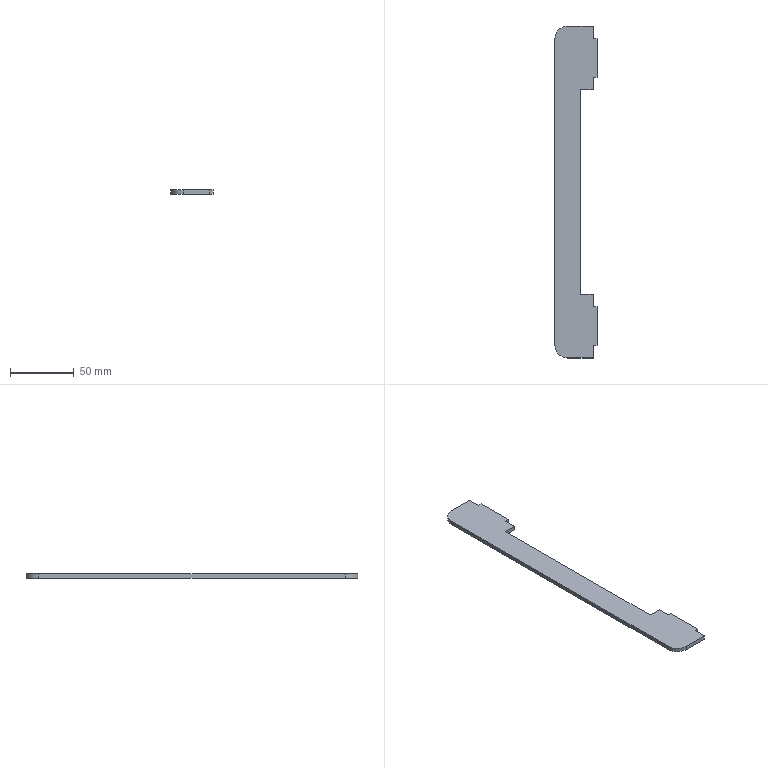Part | SolidWorks | features FlatPattern 1, SMBaseFlange 1, SheetMetal 1 | 1 solid | 20 faces | box 33 x 260 x 3.2 mm | volume 20279 mm3 | plane 18 | cylinder 2 | commonest cylinder face diameters 20 x2
STEP:
#1=CARTESIAN_POINT('',(-95.497,69.865,0.));
#2=VERTEX_POINT('',#1);
#3=CARTESIAN_POINT('',(-95.497,79.865,0.));
#4=VERTEX_POINT('',#3);
#5=CARTESIAN_POINT('',(-95.497,79.865,0.));
#6=DIRECTION('',(0.,1.,0.));
#7=VECTOR('',#6,1000.);
#8=LINE('',#5,#7);
#9=EDGE_CURVE('',#2,#4,#8,.T.);
#10=ORIENTED_EDGE('',*,*,#9,.F.);
#11=CARTESIAN_POINT('',(-95.497,69.865,-3.2));
#12=VERTEX_POINT('',#11);
#13=CARTESIAN_POINT('',(-95.497,69.865,-3.2));
#14=DIRECTION('',(0.,0.,1.));
#15=VECTOR('',#14,1000.);
#16=LINE('',#13,#15);
#17=EDGE_CURVE('',#12,#2,#16,.T.);
#18=ORIENTED_EDGE('',*,*,#17,.F.);
#19=CARTESIAN_POINT('',(-95.497,79.865,-3.2));
#20=VERTEX_POINT('',#19);
#21=CARTESIAN_POINT('',(-95.497,79.865,-3.2));
#22=DIRECTION('',(0.,1.,0.));
#23=VECTOR('',#22,1000.);
#24=LINE('',#21,#23);
#25=EDGE_CURVE('',#12,#20,#24,.T.);
#26=ORIENTED_EDGE('',*,*,#25,.T.);
#27=CARTESIAN_POINT('',(-95.497,79.865,-3.2));
#28=DIRECTION('',(0.,0.,1.));
#29=VECTOR('',#28,1000.);
#30=LINE('',#27,#29);
#31=EDGE_CURVE('',#20,#4,#30,.T.);
#32=ORIENTED_EDGE('',*,*,#31,.T.);
#33=EDGE_LOOP('',(#10,#18,#26,#32));
#34=FACE_OUTER_BOUND('',#33,.T.);
#35=CARTESIAN_POINT('',(-95.497,79.865,-3.2));
#36=DIRECTION('',(1.,0.,0.));
#37=DIRECTION('',(0.,0.,-1.));
#38=AXIS2_PLACEMENT_3D('',#35,#36,#37);
#39=PLANE('',#38);
#40=ADVANCED_FACE('',(#34),#39,.T.);
#41=CARTESIAN_POINT('',(-105.497,69.865,0.));
#42=VERTEX_POINT('',#41);
#43=CARTESIAN_POINT('',(-95.497,69.865,0.));
#44=DIRECTION('',(1.,0.,0.));
#45=VECTOR('',#44,1000.);
#46=LINE('',#43,#45);
#47=EDGE_CURVE('',#42,#2,#46,.T.);
#48=ORIENTED_EDGE('',*,*,#47,.F.);
#49=CARTESIAN_POINT('',(-105.497,69.865,-3.2));
#50=VERTEX_POINT('',#49);
#51=CARTESIAN_POINT('',(-105.497,69.865,-3.2));
#52=DIRECTION('',(0.,0.,1.));
#53=VECTOR('',#52,1000.);
#54=LINE('',#51,#53);
#55=EDGE_CURVE('',#50,#42,#54,.T.);
#56=ORIENTED_EDGE('',*,*,#55,.F.);
#57=CARTESIAN_POINT('',(-95.497,69.865,-3.2));
#58=DIRECTION('',(1.,0.,0.));
#59=VECTOR('',#58,1000.);
#60=LINE('',#57,#59);
#61=EDGE_CURVE('',#50,#12,#60,.T.);
#62=ORIENTED_EDGE('',*,*,#61,.T.);
#63=ORIENTED_EDGE('',*,*,#17,.T.);
#64=EDGE_LOOP('',(#48,#56,#62,#63));
#65=FACE_OUTER_BOUND('',#64,.T.);
#66=CARTESIAN_POINT('',(-95.497,69.865,-3.2));
#67=DIRECTION('',(0.,-1.,0.));
#68=DIRECTION('',(1.,0.,0.));
#69=AXIS2_PLACEMENT_3D('',#66,#67,#68);
#70=PLANE('',#69);
#71=ADVANCED_FACE('',(#65),#70,.T.);
#72=CARTESIAN_POINT('',(-105.497,-90.135,0.));
#73=VERTEX_POINT('',#72);
#74=CARTESIAN_POINT('',(-105.497,69.865,0.));
#75=DIRECTION('',(0.,1.,0.));
#76=VECTOR('',#75,1000.);
#77=LINE('',#74,#76);
#78=EDGE_CURVE('',#73,#42,#77,.T.);
#79=ORIENTED_EDGE('',*,*,#78,.F.);
#80=CARTESIAN_POINT('',(-105.497,-90.135,-3.2));
#81=VERTEX_POINT('',#80);
#82=CARTESIAN_POINT('',(-105.497,-90.135,-3.2));
#83=DIRECTION('',(0.,0.,1.));
#84=VECTOR('',#83,1000.);
#85=LINE('',#82,#84);
#86=EDGE_CURVE('',#81,#73,#85,.T.);
#87=ORIENTED_EDGE('',*,*,#86,.F.);
#88=CARTESIAN_POINT('',(-105.497,69.865,-3.2));
#89=DIRECTION('',(0.,1.,0.));
#90=VECTOR('',#89,1000.);
#91=LINE('',#88,#90);
#92=EDGE_CURVE('',#81,#50,#91,.T.);
#93=ORIENTED_EDGE('',*,*,#92,.T.);
#94=ORIENTED_EDGE('',*,*,#55,.T.);
#95=EDGE_LOOP('',(#79,#87,#93,#94));
#96=FACE_OUTER_BOUND('',#95,.T.);
#97=CARTESIAN_POINT('',(-105.497,69.865,-3.2));
#98=DIRECTION('',(1.,0.,0.));
#99=DIRECTION('',(0.,0.,-1.));
#100=AXIS2_PLACEMENT_3D('',#97,#98,#99);
#101=PLANE('',#100);
#102=ADVANCED_FACE('',(#96),#101,.T.);
#103=CARTESIAN_POINT('',(-95.497,-90.135,0.));
#104=VERTEX_POINT('',#103);
#105=CARTESIAN_POINT('',(-105.497,-90.135,0.));
#106=DIRECTION('',(-1.,0.,0.));
#107=VECTOR('',#106,1000.);
#108=LINE('',#105,#107);
#109=EDGE_CURVE('',#104,#73,#108,.T.);
#110=ORIENTED_EDGE('',*,*,#109,.F.);
#111=CARTESIAN_POINT('',(-95.497,-90.135,-3.2));
#112=VERTEX_POINT('',#111);
#113=CARTESIAN_POINT('',(-95.497,-90.135,-3.2));
#114=DIRECTION('',(0.,0.,1.));
#115=VECTOR('',#114,1000.);
#116=LINE('',#113,#115);
#117=EDGE_CURVE('',#112,#104,#116,.T.);
#118=ORIENTED_EDGE('',*,*,#117,.F.);
#119=CARTESIAN_POINT('',(-105.497,-90.135,-3.2));
#120=DIRECTION('',(-1.,0.,0.));
#121=VECTOR('',#120,1000.);
#122=LINE('',#119,#121);
#123=EDGE_CURVE('',#112,#81,#122,.T.);
#124=ORIENTED_EDGE('',*,*,#123,.T.);
#125=ORIENTED_EDGE('',*,*,#86,.T.);
#126=EDGE_LOOP('',(#110,#118,#124,#125));
#127=FACE_OUTER_BOUND('',#126,.T.);
#128=CARTESIAN_POINT('',(-105.497,-90.135,-3.2));
#129=DIRECTION('',(0.,1.,0.));
#130=DIRECTION('',(-1.,0.,0.));
#131=AXIS2_PLACEMENT_3D('',#128,#129,#130);
#132=PLANE('',#131);
#133=ADVANCED_FACE('',(#127),#132,.T.);
#134=CARTESIAN_POINT('',(-95.497,-100.135,0.));
#135=VERTEX_POINT('',#134);
#136=CARTESIAN_POINT('',(-95.497,-90.135,0.));
#137=DIRECTION('',(0.,1.,0.));
#138=VECTOR('',#137,1000.);
#139=LINE('',#136,#138);
#140=EDGE_CURVE('',#135,#104,#139,.T.);
#141=ORIENTED_EDGE('',*,*,#140,.F.);
#142=CARTESIAN_POINT('',(-95.497,-100.135,-3.2));
#143=VERTEX_POINT('',#142);
#144=CARTESIAN_POINT('',(-95.497,-100.135,-3.2));
#145=DIRECTION('',(0.,0.,1.));
#146=VECTOR('',#145,1000.);
#147=LINE('',#144,#146);
#148=EDGE_CURVE('',#143,#135,#147,.T.);
#149=ORIENTED_EDGE('',*,*,#148,.F.);
#150=CARTESIAN_POINT('',(-95.497,-90.135,-3.2));
#151=DIRECTION('',(0.,1.,0.));
#152=VECTOR('',#151,1000.);
#153=LINE('',#150,#152);
#154=EDGE_CURVE('',#143,#112,#153,.T.);
#155=ORIENTED_EDGE('',*,*,#154,.T.);
#156=ORIENTED_EDGE('',*,*,#117,.T.);
#157=EDGE_LOOP('',(#141,#149,#155,#156));
#158=FACE_OUTER_BOUND('',#157,.T.);
#159=CARTESIAN_POINT('',(-95.497,-90.135,-3.2));
#160=DIRECTION('',(1.,0.,0.));
#161=DIRECTION('',(0.,1.,0.));
#162=AXIS2_PLACEMENT_3D('',#159,#160,#161);
#163=PLANE('',#162);
#164=ADVANCED_FACE('',(#158),#163,.T.);
#165=CARTESIAN_POINT('',(-92.497,-100.135,0.));
#166=VERTEX_POINT('',#165);
#167=CARTESIAN_POINT('',(-95.497,-100.135,0.));
#168=DIRECTION('',(-1.,0.,0.));
#169=VECTOR('',#168,1000.);
#170=LINE('',#167,#169);
#171=EDGE_CURVE('',#166,#135,#170,.T.);
#172=ORIENTED_EDGE('',*,*,#171,.F.);
#173=CARTESIAN_POINT('',(-92.497,-100.135,-3.2));
#174=VERTEX_POINT('',#173);
#175=CARTESIAN_POINT('',(-92.497,-100.135,-3.2));
#176=DIRECTION('',(0.,0.,1.));
#177=VECTOR('',#176,1000.);
#178=LINE('',#175,#177);
#179=EDGE_CURVE('',#174,#166,#178,.T.);
#180=ORIENTED_EDGE('',*,*,#179,.F.);
#181=CARTESIAN_POINT('',(-95.497,-100.135,-3.2));
#182=DIRECTION('',(-1.,0.,0.));
#183=VECTOR('',#182,1000.);
#184=LINE('',#181,#183);
#185=EDGE_CURVE('',#174,#143,#184,.T.);
#186=ORIENTED_EDGE('',*,*,#185,.T.);
#187=ORIENTED_EDGE('',*,*,#148,.T.);
#188=EDGE_LOOP('',(#172,#180,#186,#187));
#189=FACE_OUTER_BOUND('',#188,.T.);
#190=CARTESIAN_POINT('',(-95.497,-100.135,-3.2));
#191=DIRECTION('',(0.,1.,0.));
#192=DIRECTION('',(0.,0.,1.));
#193=AXIS2_PLACEMENT_3D('',#190,#191,#192);
#194=PLANE('',#193);
#195=ADVANCED_FACE('',(#189),#194,.T.);
#196=CARTESIAN_POINT('',(-92.497,-130.135,0.));
#197=VERTEX_POINT('',#196);
#198=CARTESIAN_POINT('',(-92.497,-100.135,0.));
#199=DIRECTION('',(0.,1.,0.));
#200=VECTOR('',#199,1000.);
#201=LINE('',#198,#200);
#202=EDGE_CURVE('',#197,#166,#201,.T.);
#203=ORIENTED_EDGE('',*,*,#202,.F.);
#204=CARTESIAN_POINT('',(-92.497,-130.135,-3.2));
#205=VERTEX_POINT('',#204);
#206=CARTESIAN_POINT('',(-92.497,-130.135,-3.2));
#207=DIRECTION('',(0.,0.,1.));
#208=VECTOR('',#207,1000.);
#209=LINE('',#206,#208);
#210=EDGE_CURVE('',#205,#197,#209,.T.);
#211=ORIENTED_EDGE('',*,*,#210,.F.);
#212=CARTESIAN_POINT('',(-92.497,-100.135,-3.2));
#213=DIRECTION('',(0.,1.,0.));
#214=VECTOR('',#213,1000.);
#215=LINE('',#212,#214);
#216=EDGE_CURVE('',#205,#174,#215,.T.);
#217=ORIENTED_EDGE('',*,*,#216,.T.);
#218=ORIENTED_EDGE('',*,*,#179,.T.);
#219=EDGE_LOOP('',(#203,#211,#217,#218));
#220=FACE_OUTER_BOUND('',#219,.T.);
#221=CARTESIAN_POINT('',(-92.497,-100.135,-3.2));
#222=DIRECTION('',(1.,0.,0.));
#223=DIRECTION('',(0.,0.,-1.));
#224=AXIS2_PLACEMENT_3D('',#221,#222,#223);
#225=PLANE('',#224);
#226=ADVANCED_FACE('',(#220),#225,.T.);
#227=CARTESIAN_POINT('',(-95.497,-130.135,0.));
#228=VERTEX_POINT('',#227);
#229=CARTESIAN_POINT('',(-92.497,-130.135,0.));
#230=DIRECTION('',(1.,0.,0.));
#231=VECTOR('',#230,1000.);
#232=LINE('',#229,#231);
#233=EDGE_CURVE('',#228,#197,#232,.T.);
#234=ORIENTED_EDGE('',*,*,#233,.F.);
#235=CARTESIAN_POINT('',(-95.497,-130.135,-3.2));
#236=VERTEX_POINT('',#235);
#237=CARTESIAN_POINT('',(-95.497,-130.135,-3.2));
#238=DIRECTION('',(0.,0.,1.));
#239=VECTOR('',#238,1000.);
#240=LINE('',#237,#239);
#241=EDGE_CURVE('',#236,#228,#240,.T.);
#242=ORIENTED_EDGE('',*,*,#241,.F.);
#243=CARTESIAN_POINT('',(-92.497,-130.135,-3.2));
#244=DIRECTION('',(1.,0.,0.));
#245=VECTOR('',#244,1000.);
#246=LINE('',#243,#245);
#247=EDGE_CURVE('',#236,#205,#246,.T.);
#248=ORIENTED_EDGE('',*,*,#247,.T.);
#249=ORIENTED_EDGE('',*,*,#210,.T.);
#250=EDGE_LOOP('',(#234,#242,#248,#249));
#251=FACE_OUTER_BOUND('',#250,.T.);
#252=CARTESIAN_POINT('',(-92.497,-130.135,-3.2));
#253=DIRECTION('',(0.,-1.,0.));
#254=DIRECTION('',(0.,0.,-1.));
#255=AXIS2_PLACEMENT_3D('',#252,#253,#254);
#256=PLANE('',#255);
#257=ADVANCED_FACE('',(#251),#256,.T.);
#258=CARTESIAN_POINT('',(-95.497,-140.135,0.));
#259=VERTEX_POINT('',#258);
#260=CARTESIAN_POINT('',(-95.497,-130.135,0.));
#261=DIRECTION('',(0.,1.,0.));
#262=VECTOR('',#261,1000.);
#263=LINE('',#260,#262);
#264=EDGE_CURVE('',#259,#228,#263,.T.);
#265=ORIENTED_EDGE('',*,*,#264,.F.);
#266=CARTESIAN_POINT('',(-95.497,-140.135,-3.2));
#267=VERTEX_POINT('',#266);
#268=CARTESIAN_POINT('',(-95.497,-140.135,-3.2));
#269=DIRECTION('',(0.,0.,1.));
#270=VECTOR('',#269,1000.);
#271=LINE('',#268,#270);
#272=EDGE_CURVE('',#267,#259,#271,.T.);
#273=ORIENTED_EDGE('',*,*,#272,.F.);
#274=CARTESIAN_POINT('',(-95.497,-130.135,-3.2));
#275=DIRECTION('',(0.,1.,0.));
#276=VECTOR('',#275,1000.);
#277=LINE('',#274,#276);
#278=EDGE_CURVE('',#267,#236,#277,.T.);
#279=ORIENTED_EDGE('',*,*,#278,.T.);
#280=ORIENTED_EDGE('',*,*,#241,.T.);
#281=EDGE_LOOP('',(#265,#273,#279,#280));
#282=FACE_OUTER_BOUND('',#281,.T.);
#283=CARTESIAN_POINT('',(-95.497,-130.135,-3.2));
#284=DIRECTION('',(1.,0.,0.));
#285=DIRECTION('',(0.,1.,0.));
#286=AXIS2_PLACEMENT_3D('',#283,#284,#285);
#287=PLANE('',#286);
#288=ADVANCED_FACE('',(#282),#287,.T.);
#289=CARTESIAN_POINT('',(-115.497,-140.135,0.));
#290=VERTEX_POINT('',#289);
#291=CARTESIAN_POINT('',(-95.497,-140.135,0.));
#292=DIRECTION('',(1.,0.,0.));
#293=VECTOR('',#292,1000.);
#294=LINE('',#291,#293);
#295=EDGE_CURVE('',#290,#259,#294,.T.);
#296=ORIENTED_EDGE('',*,*,#295,.F.);
#297=CARTESIAN_POINT('',(-115.497,-140.135,-3.2));
#298=VERTEX_POINT('',#297);
#299=CARTESIAN_POINT('',(-115.497,-140.135,-3.2));
#300=DIRECTION('',(0.,0.,1.));
#301=VECTOR('',#300,1000.);
#302=LINE('',#299,#301);
#303=EDGE_CURVE('',#298,#290,#302,.T.);
#304=ORIENTED_EDGE('',*,*,#303,.F.);
#305=CARTESIAN_POINT('',(-95.497,-140.135,-3.2));
#306=DIRECTION('',(1.,0.,0.));
#307=VECTOR('',#306,1000.);
#308=LINE('',#305,#307);
#309=EDGE_CURVE('',#298,#267,#308,.T.);
#310=ORIENTED_EDGE('',*,*,#309,.T.);
#311=ORIENTED_EDGE('',*,*,#272,.T.);
#312=EDGE_LOOP('',(#296,#304,#310,#311));
#313=FACE_OUTER_BOUND('',#312,.T.);
#314=CARTESIAN_POINT('',(-95.497,-140.135,-3.2));
#315=DIRECTION('',(0.,-1.,0.));
#316=DIRECTION('',(0.,0.,-1.));
#317=AXIS2_PLACEMENT_3D('',#314,#315,#316);
#318=PLANE('',#317);
#319=ADVANCED_FACE('',(#313),#318,.T.);
#320=CARTESIAN_POINT('',(-125.497,-130.135,0.));
#321=VERTEX_POINT('',#320);
#322=CARTESIAN_POINT('',(-115.497,-130.135,0.));
#323=DIRECTION('',(0.,0.,1.));
#324=DIRECTION('',(-1.,0.,0.));
#325=AXIS2_PLACEMENT_3D('',#322,#323,#324);
#326=CIRCLE('',#325,10.);
#327=EDGE_CURVE('',#321,#290,#326,.T.);
#328=ORIENTED_EDGE('',*,*,#327,.F.);
#329=CARTESIAN_POINT('',(-125.497,-130.135,-3.2));
#330=VERTEX_POINT('',#329);
#331=CARTESIAN_POINT('',(-125.497,-130.135,-3.2));
#332=DIRECTION('',(0.,0.,1.));
#333=VECTOR('',#332,1000.);
#334=LINE('',#331,#333);
#335=EDGE_CURVE('',#330,#321,#334,.T.);
#336=ORIENTED_EDGE('',*,*,#335,.F.);
#337=CARTESIAN_POINT('',(-115.497,-130.135,-3.2));
#338=DIRECTION('',(0.,0.,1.));
#339=DIRECTION('',(-1.,0.,0.));
#340=AXIS2_PLACEMENT_3D('',#337,#338,#339);
#341=CIRCLE('',#340,10.);
#342=EDGE_CURVE('',#330,#298,#341,.T.);
#343=ORIENTED_EDGE('',*,*,#342,.T.);
#344=ORIENTED_EDGE('',*,*,#303,.T.);
#345=EDGE_LOOP('',(#328,#336,#343,#344));
#346=FACE_OUTER_BOUND('',#345,.T.);
#347=CARTESIAN_POINT('',(-115.497,-130.135,-3.2));
#348=DIRECTION('',(0.,0.,1.));
#349=DIRECTION('',(1.,0.,0.));
#350=AXIS2_PLACEMENT_3D('',#347,#348,#349);
#351=CYLINDRICAL_SURFACE('',#350,10.);
#352=ADVANCED_FACE('',(#346),#351,.T.);
#353=CARTESIAN_POINT('',(-125.497,109.865,0.));
#354=VERTEX_POINT('',#353);
#355=CARTESIAN_POINT('',(-125.497,-130.135,0.));
#356=DIRECTION('',(0.,-1.,0.));
#357=VECTOR('',#356,1000.);
#358=LINE('',#355,#357);
#359=EDGE_CURVE('',#354,#321,#358,.T.);
#360=ORIENTED_EDGE('',*,*,#359,.F.);
#361=CARTESIAN_POINT('',(-125.497,109.865,-3.2));
#362=VERTEX_POINT('',#361);
#363=CARTESIAN_POINT('',(-125.497,109.865,-3.2));
#364=DIRECTION('',(0.,0.,1.));
#365=VECTOR('',#364,1000.);
#366=LINE('',#363,#365);
#367=EDGE_CURVE('',#362,#354,#366,.T.);
#368=ORIENTED_EDGE('',*,*,#367,.F.);
#369=CARTESIAN_POINT('',(-125.497,-130.135,-3.2));
#370=DIRECTION('',(0.,-1.,0.));
#371=VECTOR('',#370,1000.);
#372=LINE('',#369,#371);
#373=EDGE_CURVE('',#362,#330,#372,.T.);
#374=ORIENTED_EDGE('',*,*,#373,.T.);
#375=ORIENTED_EDGE('',*,*,#335,.T.);
#376=EDGE_LOOP('',(#360,#368,#374,#375));
#377=FACE_OUTER_BOUND('',#376,.T.);
#378=CARTESIAN_POINT('',(-125.497,-130.135,-3.2));
#379=DIRECTION('',(-1.,0.,0.));
#380=DIRECTION('',(0.,0.,1.));
#381=AXIS2_PLACEMENT_3D('',#378,#379,#380);
#382=PLANE('',#381);
#383=ADVANCED_FACE('',(#377),#382,.T.);
#384=CARTESIAN_POINT('',(-115.497,119.865,0.));
#385=VERTEX_POINT('',#384);
#386=CARTESIAN_POINT('',(-115.497,109.865,0.));
#387=DIRECTION('',(0.,0.,1.));
#388=DIRECTION('',(-1.,0.,0.));
#389=AXIS2_PLACEMENT_3D('',#386,#387,#388);
#390=CIRCLE('',#389,10.);
#391=EDGE_CURVE('',#385,#354,#390,.T.);
#392=ORIENTED_EDGE('',*,*,#391,.F.);
#393=CARTESIAN_POINT('',(-115.497,119.865,-3.2));
#394=VERTEX_POINT('',#393);
#395=CARTESIAN_POINT('',(-115.497,119.865,-3.2));
#396=DIRECTION('',(0.,0.,1.));
#397=VECTOR('',#396,1000.);
#398=LINE('',#395,#397);
#399=EDGE_CURVE('',#394,#385,#398,.T.);
#400=ORIENTED_EDGE('',*,*,#399,.F.);
#401=CARTESIAN_POINT('',(-115.497,109.865,-3.2));
#402=DIRECTION('',(0.,0.,1.));
#403=DIRECTION('',(-1.,0.,0.));
#404=AXIS2_PLACEMENT_3D('',#401,#402,#403);
#405=CIRCLE('',#404,10.);
#406=EDGE_CURVE('',#394,#362,#405,.T.);
#407=ORIENTED_EDGE('',*,*,#406,.T.);
#408=ORIENTED_EDGE('',*,*,#367,.T.);
#409=EDGE_LOOP('',(#392,#400,#407,#408));
#410=FACE_OUTER_BOUND('',#409,.T.);
#411=CARTESIAN_POINT('',(-115.497,109.865,-3.2));
#412=DIRECTION('',(0.,0.,1.));
#413=DIRECTION('',(1.,0.,0.));
#414=AXIS2_PLACEMENT_3D('',#411,#412,#413);
#415=CYLINDRICAL_SURFACE('',#414,10.);
#416=ADVANCED_FACE('',(#410),#415,.T.);
#417=CARTESIAN_POINT('',(-95.497,119.865,0.));
#418=VERTEX_POINT('',#417);
#419=CARTESIAN_POINT('',(-115.497,119.865,0.));
#420=DIRECTION('',(-1.,0.,0.));
#421=VECTOR('',#420,1000.);
#422=LINE('',#419,#421);
#423=EDGE_CURVE('',#418,#385,#422,.T.);
#424=ORIENTED_EDGE('',*,*,#423,.F.);
#425=CARTESIAN_POINT('',(-95.497,119.865,-3.2));
#426=VERTEX_POINT('',#425);
#427=CARTESIAN_POINT('',(-95.497,119.865,-3.2));
#428=DIRECTION('',(0.,0.,1.));
#429=VECTOR('',#428,1000.);
#430=LINE('',#427,#429);
#431=EDGE_CURVE('',#426,#418,#430,.T.);
#432=ORIENTED_EDGE('',*,*,#431,.F.);
#433=CARTESIAN_POINT('',(-115.497,119.865,-3.2));
#434=DIRECTION('',(-1.,0.,0.));
#435=VECTOR('',#434,1000.);
#436=LINE('',#433,#435);
#437=EDGE_CURVE('',#426,#394,#436,.T.);
#438=ORIENTED_EDGE('',*,*,#437,.T.);
#439=ORIENTED_EDGE('',*,*,#399,.T.);
#440=EDGE_LOOP('',(#424,#432,#438,#439));
#441=FACE_OUTER_BOUND('',#440,.T.);
#442=CARTESIAN_POINT('',(-115.497,119.865,-3.2));
#443=DIRECTION('',(0.,1.,0.));
#444=DIRECTION('',(0.,0.,1.));
#445=AXIS2_PLACEMENT_3D('',#442,#443,#444);
#446=PLANE('',#445);
#447=ADVANCED_FACE('',(#441),#446,.T.);
#448=CARTESIAN_POINT('',(-95.497,109.865,0.));
#449=VERTEX_POINT('',#448);
#450=CARTESIAN_POINT('',(-95.497,119.865,0.));
#451=DIRECTION('',(0.,1.,0.));
#452=VECTOR('',#451,1000.);
#453=LINE('',#450,#452);
#454=EDGE_CURVE('',#449,#418,#453,.T.);
#455=ORIENTED_EDGE('',*,*,#454,.F.);
#456=CARTESIAN_POINT('',(-95.497,109.865,-3.2));
#457=VERTEX_POINT('',#456);
#458=CARTESIAN_POINT('',(-95.497,109.865,-3.2));
#459=DIRECTION('',(0.,0.,1.));
#460=VECTOR('',#459,1000.);
#461=LINE('',#458,#460);
#462=EDGE_CURVE('',#457,#449,#461,.T.);
#463=ORIENTED_EDGE('',*,*,#462,.F.);
#464=CARTESIAN_POINT('',(-95.497,119.865,-3.2));
#465=DIRECTION('',(0.,1.,0.));
#466=VECTOR('',#465,1000.);
#467=LINE('',#464,#466);
#468=EDGE_CURVE('',#457,#426,#467,.T.);
#469=ORIENTED_EDGE('',*,*,#468,.T.);
#470=ORIENTED_EDGE('',*,*,#431,.T.);
#471=EDGE_LOOP('',(#455,#463,#469,#470));
#472=FACE_OUTER_BOUND('',#471,.T.);
#473=CARTESIAN_POINT('',(-95.497,119.865,-3.2));
#474=DIRECTION('',(1.,0.,0.));
#475=DIRECTION('',(0.,1.,0.));
#476=AXIS2_PLACEMENT_3D('',#473,#474,#475);
#477=PLANE('',#476);
#478=ADVANCED_FACE('',(#472),#477,.T.);
#479=CARTESIAN_POINT('',(-92.497,109.865,0.));
#480=VERTEX_POINT('',#479);
#481=CARTESIAN_POINT('',(-95.497,109.865,0.));
#482=DIRECTION('',(-1.,0.,0.));
#483=VECTOR('',#482,1000.);
#484=LINE('',#481,#483);
#485=EDGE_CURVE('',#480,#449,#484,.T.);
#486=ORIENTED_EDGE('',*,*,#485,.F.);
#487=CARTESIAN_POINT('',(-92.497,109.865,-3.2));
#488=VERTEX_POINT('',#487);
#489=CARTESIAN_POINT('',(-92.497,109.865,-3.2));
#490=DIRECTION('',(0.,0.,1.));
#491=VECTOR('',#490,1000.);
#492=LINE('',#489,#491);
#493=EDGE_CURVE('',#488,#480,#492,.T.);
#494=ORIENTED_EDGE('',*,*,#493,.F.);
#495=CARTESIAN_POINT('',(-95.497,109.865,-3.2));
#496=DIRECTION('',(-1.,0.,0.));
#497=VECTOR('',#496,1000.);
#498=LINE('',#495,#497);
#499=EDGE_CURVE('',#488,#457,#498,.T.);
#500=ORIENTED_EDGE('',*,*,#499,.T.);
#501=ORIENTED_EDGE('',*,*,#462,.T.);
#502=EDGE_LOOP('',(#486,#494,#500,#501));
#503=FACE_OUTER_BOUND('',#502,.T.);
#504=CARTESIAN_POINT('',(-95.497,109.865,-3.2));
#505=DIRECTION('',(0.,1.,0.));
#506=DIRECTION('',(0.,0.,1.));
#507=AXIS2_PLACEMENT_3D('',#504,#505,#506);
#508=PLANE('',#507);
#509=ADVANCED_FACE('',(#503),#508,.T.);
#510=CARTESIAN_POINT('',(-92.497,79.865,0.));
#511=VERTEX_POINT('',#510);
#512=CARTESIAN_POINT('',(-92.497,109.865,0.));
#513=DIRECTION('',(0.,1.,0.));
#514=VECTOR('',#513,1000.);
#515=LINE('',#512,#514);
#516=EDGE_CURVE('',#511,#480,#515,.T.);
#517=ORIENTED_EDGE('',*,*,#516,.F.);
#518=CARTESIAN_POINT('',(-92.497,79.865,-3.2));
#519=VERTEX_POINT('',#518);
#520=CARTESIAN_POINT('',(-92.497,79.865,-3.2));
#521=DIRECTION('',(0.,0.,1.));
#522=VECTOR('',#521,1000.);
#523=LINE('',#520,#522);
#524=EDGE_CURVE('',#519,#511,#523,.T.);
#525=ORIENTED_EDGE('',*,*,#524,.F.);
#526=CARTESIAN_POINT('',(-92.497,109.865,-3.2));
#527=DIRECTION('',(0.,1.,0.));
#528=VECTOR('',#527,1000.);
#529=LINE('',#526,#528);
#530=EDGE_CURVE('',#519,#488,#529,.T.);
#531=ORIENTED_EDGE('',*,*,#530,.T.);
#532=ORIENTED_EDGE('',*,*,#493,.T.);
#533=EDGE_LOOP('',(#517,#525,#531,#532));
#534=FACE_OUTER_BOUND('',#533,.T.);
#535=CARTESIAN_POINT('',(-92.497,109.865,-3.2));
#536=DIRECTION('',(1.,0.,0.));
#537=DIRECTION('',(0.,0.,-1.));
#538=AXIS2_PLACEMENT_3D('',#535,#536,#537);
#539=PLANE('',#538);
#540=ADVANCED_FACE('',(#534),#539,.T.);
#541=CARTESIAN_POINT('',(-92.497,79.865,0.));
#542=DIRECTION('',(1.,0.,0.));
#543=VECTOR('',#542,1000.);
#544=LINE('',#541,#543);
#545=EDGE_CURVE('',#4,#511,#544,.T.);
#546=ORIENTED_EDGE('',*,*,#545,.F.);
#547=ORIENTED_EDGE('',*,*,#31,.F.);
#548=CARTESIAN_POINT('',(-92.497,79.865,-3.2));
#549=DIRECTION('',(1.,0.,0.));
#550=VECTOR('',#549,1000.);
#551=LINE('',#548,#550);
#552=EDGE_CURVE('',#20,#519,#551,.T.);
#553=ORIENTED_EDGE('',*,*,#552,.T.);
#554=ORIENTED_EDGE('',*,*,#524,.T.);
#555=EDGE_LOOP('',(#546,#547,#553,#554));
#556=FACE_OUTER_BOUND('',#555,.T.);
#557=CARTESIAN_POINT('',(-92.497,79.865,-3.2));
#558=DIRECTION('',(0.,-1.,0.));
#559=DIRECTION('',(0.,0.,-1.));
#560=AXIS2_PLACEMENT_3D('',#557,#558,#559);
#561=PLANE('',#560);
#562=ADVANCED_FACE('',(#556),#561,.T.);
#563=ORIENTED_EDGE('',*,*,#25,.F.);
#564=ORIENTED_EDGE('',*,*,#61,.F.);
#565=ORIENTED_EDGE('',*,*,#92,.F.);
#566=ORIENTED_EDGE('',*,*,#123,.F.);
#567=ORIENTED_EDGE('',*,*,#154,.F.);
#568=ORIENTED_EDGE('',*,*,#185,.F.);
#569=ORIENTED_EDGE('',*,*,#216,.F.);
#570=ORIENTED_EDGE('',*,*,#247,.F.);
#571=ORIENTED_EDGE('',*,*,#278,.F.);
#572=ORIENTED_EDGE('',*,*,#309,.F.);
#573=ORIENTED_EDGE('',*,*,#342,.F.);
#574=ORIENTED_EDGE('',*,*,#373,.F.);
#575=ORIENTED_EDGE('',*,*,#406,.F.);
#576=ORIENTED_EDGE('',*,*,#437,.F.);
#577=ORIENTED_EDGE('',*,*,#468,.F.);
#578=ORIENTED_EDGE('',*,*,#499,.F.);
#579=ORIENTED_EDGE('',*,*,#530,.F.);
#580=ORIENTED_EDGE('',*,*,#552,.F.);
#581=EDGE_LOOP('',(#563,#564,#565,#566,#567,#568,#569,#570,#571,#572,#573,#574,#575,#576,#577,#578,#579,#580));
#582=FACE_OUTER_BOUND('',#581,.T.);
#583=CARTESIAN_POINT('',(-115.497,-130.135,-3.2));
#584=DIRECTION('',(0.,0.,-1.));
#585=DIRECTION('',(-1.,0.,0.));
#586=AXIS2_PLACEMENT_3D('',#583,#584,#585);
#587=PLANE('',#586);
#588=ADVANCED_FACE('',(#582),#587,.T.);
#589=ORIENTED_EDGE('',*,*,#9,.T.);
#590=ORIENTED_EDGE('',*,*,#545,.T.);
#591=ORIENTED_EDGE('',*,*,#516,.T.);
#592=ORIENTED_EDGE('',*,*,#485,.T.);
#593=ORIENTED_EDGE('',*,*,#454,.T.);
#594=ORIENTED_EDGE('',*,*,#423,.T.);
#595=ORIENTED_EDGE('',*,*,#391,.T.);
#596=ORIENTED_EDGE('',*,*,#359,.T.);
#597=ORIENTED_EDGE('',*,*,#327,.T.);
#598=ORIENTED_EDGE('',*,*,#295,.T.);
#599=ORIENTED_EDGE('',*,*,#264,.T.);
#600=ORIENTED_EDGE('',*,*,#233,.T.);
#601=ORIENTED_EDGE('',*,*,#202,.T.);
#602=ORIENTED_EDGE('',*,*,#171,.T.);
#603=ORIENTED_EDGE('',*,*,#140,.T.);
#604=ORIENTED_EDGE('',*,*,#109,.T.);
#605=ORIENTED_EDGE('',*,*,#78,.T.);
#606=ORIENTED_EDGE('',*,*,#47,.T.);
#607=EDGE_LOOP('',(#589,#590,#591,#592,#593,#594,#595,#596,#597,#598,#599,#600,#601,#602,#603,#604,#605,#606));
#608=FACE_OUTER_BOUND('',#607,.T.);
#609=CARTESIAN_POINT('',(-115.497,-130.135,0.));
#610=DIRECTION('',(0.,0.,-1.));
#611=DIRECTION('',(-1.,0.,0.));
#612=AXIS2_PLACEMENT_3D('',#609,#610,#611);
#613=PLANE('',#612);
#614=ADVANCED_FACE('',(#608),#613,.F.);
#615=CLOSED_SHELL('',(#40,#71,#102,#133,#164,#195,#226,#257,#288,#319,#352,#383,#416,#447,#478,#509,#540,#562,#588,#614));
#616=MANIFOLD_SOLID_BREP('',#615);
#617=CARTESIAN_POINT('',(0.,0.,0.));
#618=DIRECTION('',(0.,0.,1.));
#619=DIRECTION('',(1.,0.,0.));
#620=AXIS2_PLACEMENT_3D('',#617,#618,#619);
#621=(LENGTH_UNIT()NAMED_UNIT(*)SI_UNIT(.MILLI.,.METRE.));
#622=UNCERTAINTY_MEASURE_WITH_UNIT(LENGTH_MEASURE(0.00001),#621,'','');
#623=(NAMED_UNIT(*)PLANE_ANGLE_UNIT()SI_UNIT($,.RADIAN.));
#624=(NAMED_UNIT(*)SI_UNIT($,.STERADIAN.)SOLID_ANGLE_UNIT());
#625=(GEOMETRIC_REPRESENTATION_CONTEXT(3)GLOBAL_UNCERTAINTY_ASSIGNED_CONTEXT((#622))GLOBAL_UNIT_ASSIGNED_CONTEXT((#621,#623,#624))REPRESENTATION_CONTEXT('',''));
#626=ADVANCED_BREP_SHAPE_REPRESENTATION('',(#616,#620),#625);